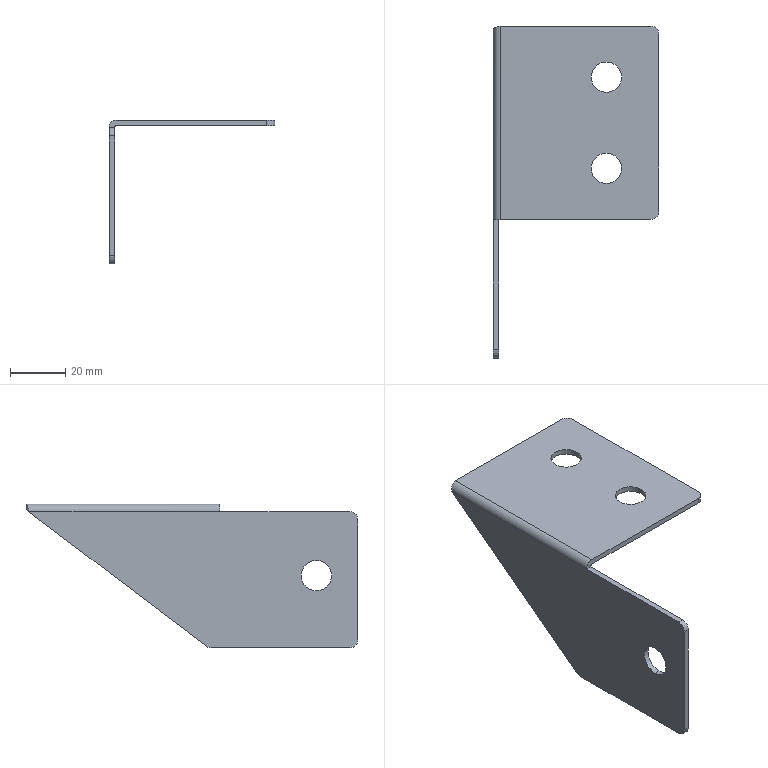Part | SolidWorks | features BaseBody 1 | 1 solid | 25 faces | box 60 x 120 x 52 mm | volume 16335 mm3 | cylinder 13 | plane 11 | spline 1 | commonest cylinder face diameters 11 x6 6 x5 1.473 x1 5.473 x1
STEP:
#1=CARTESIAN_POINT('',(-28.,-70.,-53.368));
#2=VERTEX_POINT('',#1);
#3=CARTESIAN_POINT('',(-28.,-70.,-42.368));
#4=VERTEX_POINT('',#3);
#5=CARTESIAN_POINT('',(-28.,-70.,-47.868));
#6=DIRECTION('',(-1.,0.,0.));
#7=DIRECTION('',(0.,0.,1.));
#8=AXIS2_PLACEMENT_3D('',#5,#6,#7);
#9=CIRCLE('',#8,5.5);
#10=EDGE_CURVE('',#2,#4,#9,.T.);
#11=ORIENTED_EDGE('',*,*,#10,.F.);
#12=CARTESIAN_POINT('',(-30.,-70.,-53.368));
#13=VERTEX_POINT('',#12);
#14=CARTESIAN_POINT('',(-20.,-70.,-53.368));
#15=DIRECTION('',(-1.,0.,0.));
#16=VECTOR('',#15,1000.);
#17=LINE('',#14,#16);
#18=EDGE_CURVE('',#2,#13,#17,.T.);
#19=ORIENTED_EDGE('',*,*,#18,.T.);
#20=CARTESIAN_POINT('',(-30.,-70.,-42.368));
#21=VERTEX_POINT('',#20);
#22=CARTESIAN_POINT('',(-30.,-70.,-47.868));
#23=DIRECTION('',(1.,0.,0.));
#24=DIRECTION('',(0.,0.,1.));
#25=AXIS2_PLACEMENT_3D('',#22,#23,#24);
#26=CIRCLE('',#25,5.5);
#27=EDGE_CURVE('',#21,#13,#26,.T.);
#28=ORIENTED_EDGE('',*,*,#27,.F.);
#29=CARTESIAN_POINT('',(-20.,-70.,-42.368));
#30=DIRECTION('',(-1.,0.,0.));
#31=VECTOR('',#30,1000.);
#32=LINE('',#29,#31);
#33=EDGE_CURVE('',#4,#21,#32,.T.);
#34=ORIENTED_EDGE('',*,*,#33,.F.);
#35=EDGE_LOOP('',(#11,#19,#28,#34));
#36=FACE_OUTER_BOUND('',#35,.T.);
#37=CARTESIAN_POINT('',(-20.,-70.,-47.868));
#38=DIRECTION('',(-1.,0.,0.));
#39=DIRECTION('',(0.,0.,1.));
#40=AXIS2_PLACEMENT_3D('',#37,#38,#39);
#41=CYLINDRICAL_SURFACE('',#40,5.5);
#42=ADVANCED_FACE('',(#36),#41,.F.);
#43=CARTESIAN_POINT('',(16.5,16.5,-22.));
#44=VERTEX_POINT('',#43);
#45=CARTESIAN_POINT('',(5.5,16.5,-22.));
#46=VERTEX_POINT('',#45);
#47=CARTESIAN_POINT('',(11.,16.5,-22.));
#48=DIRECTION('',(0.,0.,-1.));
#49=DIRECTION('',(-1.,0.,0.));
#50=AXIS2_PLACEMENT_3D('',#47,#48,#49);
#51=CIRCLE('',#50,5.5);
#52=EDGE_CURVE('',#44,#46,#51,.T.);
#53=ORIENTED_EDGE('',*,*,#52,.F.);
#54=CARTESIAN_POINT('',(16.5,16.5,-24.));
#55=VERTEX_POINT('',#54);
#56=CARTESIAN_POINT('',(16.5,16.5,-22.));
#57=DIRECTION('',(0.,0.,-1.));
#58=VECTOR('',#57,1000.);
#59=LINE('',#56,#58);
#60=EDGE_CURVE('',#44,#55,#59,.T.);
#61=ORIENTED_EDGE('',*,*,#60,.T.);
#62=CARTESIAN_POINT('',(5.5,16.5,-24.));
#63=VERTEX_POINT('',#62);
#64=CARTESIAN_POINT('',(11.,16.5,-24.));
#65=DIRECTION('',(0.,0.,1.));
#66=DIRECTION('',(-1.,0.,0.));
#67=AXIS2_PLACEMENT_3D('',#64,#65,#66);
#68=CIRCLE('',#67,5.5);
#69=EDGE_CURVE('',#63,#55,#68,.T.);
#70=ORIENTED_EDGE('',*,*,#69,.F.);
#71=CARTESIAN_POINT('',(5.5,16.5,-22.));
#72=DIRECTION('',(0.,0.,-1.));
#73=VECTOR('',#72,1000.);
#74=LINE('',#71,#73);
#75=EDGE_CURVE('',#46,#63,#74,.T.);
#76=ORIENTED_EDGE('',*,*,#75,.F.);
#77=EDGE_LOOP('',(#53,#61,#70,#76));
#78=FACE_OUTER_BOUND('',#77,.T.);
#79=CARTESIAN_POINT('',(11.,16.5,-22.));
#80=DIRECTION('',(0.,0.,-1.));
#81=DIRECTION('',(-1.,0.,0.));
#82=AXIS2_PLACEMENT_3D('',#79,#80,#81);
#83=CYLINDRICAL_SURFACE('',#82,5.5);
#84=ADVANCED_FACE('',(#78),#83,.F.);
#85=CARTESIAN_POINT('',(16.5,-16.5,-22.));
#86=VERTEX_POINT('',#85);
#87=CARTESIAN_POINT('',(5.5,-16.5,-22.));
#88=VERTEX_POINT('',#87);
#89=CARTESIAN_POINT('',(11.,-16.5,-22.));
#90=DIRECTION('',(0.,0.,-1.));
#91=DIRECTION('',(-1.,0.,0.));
#92=AXIS2_PLACEMENT_3D('',#89,#90,#91);
#93=CIRCLE('',#92,5.5);
#94=EDGE_CURVE('',#86,#88,#93,.T.);
#95=ORIENTED_EDGE('',*,*,#94,.F.);
#96=CARTESIAN_POINT('',(16.5,-16.5,-24.));
#97=VERTEX_POINT('',#96);
#98=CARTESIAN_POINT('',(16.5,-16.5,-22.));
#99=DIRECTION('',(0.,0.,-1.));
#100=VECTOR('',#99,1000.);
#101=LINE('',#98,#100);
#102=EDGE_CURVE('',#86,#97,#101,.T.);
#103=ORIENTED_EDGE('',*,*,#102,.T.);
#104=CARTESIAN_POINT('',(5.5,-16.5,-24.));
#105=VERTEX_POINT('',#104);
#106=CARTESIAN_POINT('',(11.,-16.5,-24.));
#107=DIRECTION('',(0.,0.,1.));
#108=DIRECTION('',(-1.,0.,0.));
#109=AXIS2_PLACEMENT_3D('',#106,#107,#108);
#110=CIRCLE('',#109,5.5);
#111=EDGE_CURVE('',#105,#97,#110,.T.);
#112=ORIENTED_EDGE('',*,*,#111,.F.);
#113=CARTESIAN_POINT('',(5.5,-16.5,-22.));
#114=DIRECTION('',(0.,0.,-1.));
#115=VECTOR('',#114,1000.);
#116=LINE('',#113,#115);
#117=EDGE_CURVE('',#88,#105,#116,.T.);
#118=ORIENTED_EDGE('',*,*,#117,.F.);
#119=EDGE_LOOP('',(#95,#103,#112,#118));
#120=FACE_OUTER_BOUND('',#119,.T.);
#121=CARTESIAN_POINT('',(11.,-16.5,-22.));
#122=DIRECTION('',(0.,0.,-1.));
#123=DIRECTION('',(-1.,0.,0.));
#124=AXIS2_PLACEMENT_3D('',#121,#122,#123);
#125=CYLINDRICAL_SURFACE('',#124,5.5);
#126=ADVANCED_FACE('',(#120),#125,.F.);
#127=CARTESIAN_POINT('',(-30.,-32.,-74.));
#128=VERTEX_POINT('',#127);
#129=CARTESIAN_POINT('',(-30.,-82.,-74.));
#130=VERTEX_POINT('',#129);
#131=CARTESIAN_POINT('',(-30.,-32.,-74.));
#132=DIRECTION('',(0.,-1.,0.));
#133=VECTOR('',#132,1000.);
#134=LINE('',#131,#133);
#135=EDGE_CURVE('',#128,#130,#134,.T.);
#136=ORIENTED_EDGE('',*,*,#135,.T.);
#137=CARTESIAN_POINT('',(-30.,-85.,-71.));
#138=VERTEX_POINT('',#137);
#139=CARTESIAN_POINT('',(-30.,-82.,-71.));
#140=DIRECTION('',(-1.,0.,0.));
#141=DIRECTION('',(0.,0.,-1.));
#142=AXIS2_PLACEMENT_3D('',#139,#140,#141);
#143=CIRCLE('',#142,3.);
#144=EDGE_CURVE('',#130,#138,#143,.T.);
#145=ORIENTED_EDGE('',*,*,#144,.T.);
#146=CARTESIAN_POINT('',(-30.,-85.,-27.737));
#147=VERTEX_POINT('',#146);
#148=CARTESIAN_POINT('',(-30.,-85.,-71.));
#149=DIRECTION('',(0.,0.,1.));
#150=VECTOR('',#149,1000.);
#151=LINE('',#148,#150);
#152=EDGE_CURVE('',#138,#147,#151,.T.);
#153=ORIENTED_EDGE('',*,*,#152,.T.);
#154=CARTESIAN_POINT('',(-30.,-82.,-24.737));
#155=VERTEX_POINT('',#154);
#156=CARTESIAN_POINT('',(-30.,-82.,-27.737));
#157=DIRECTION('',(-1.,0.,0.));
#158=DIRECTION('',(0.,0.,-1.));
#159=AXIS2_PLACEMENT_3D('',#156,#157,#158);
#160=CIRCLE('',#159,3.);
#161=EDGE_CURVE('',#147,#155,#160,.T.);
#162=ORIENTED_EDGE('',*,*,#161,.T.);
#163=CARTESIAN_POINT('',(-30.,-35.,-24.737));
#164=VERTEX_POINT('',#163);
#165=CARTESIAN_POINT('',(-30.,-32.,-24.737));
#166=DIRECTION('',(0.,1.,0.));
#167=VECTOR('',#166,1000.);
#168=LINE('',#165,#167);
#169=EDGE_CURVE('',#155,#164,#168,.T.);
#170=ORIENTED_EDGE('',*,*,#169,.T.);
#171=CARTESIAN_POINT('',(-30.,34.028,-24.737));
#172=VERTEX_POINT('',#171);
#173=CARTESIAN_POINT('',(-30.,-32.,-24.737));
#174=DIRECTION('',(0.,1.,0.));
#175=VECTOR('',#174,1000.);
#176=LINE('',#173,#175);
#177=EDGE_CURVE('',#164,#172,#176,.T.);
#178=ORIENTED_EDGE('',*,*,#177,.T.);
#179=CARTESIAN_POINT('',(-30.,-30.188,-73.391));
#180=VERTEX_POINT('',#179);
#181=CARTESIAN_POINT('',(-30.,34.028,-24.737));
#182=DIRECTION('',(0.,-0.7971,-0.6039));
#183=VECTOR('',#182,1000.);
#184=LINE('',#181,#183);
#185=EDGE_CURVE('',#172,#180,#184,.T.);
#186=ORIENTED_EDGE('',*,*,#185,.T.);
#187=CARTESIAN_POINT('',(-30.,-32.,-71.));
#188=DIRECTION('',(-1.,0.,0.));
#189=DIRECTION('',(0.,0.,-1.));
#190=AXIS2_PLACEMENT_3D('',#187,#188,#189);
#191=CIRCLE('',#190,3.);
#192=EDGE_CURVE('',#180,#128,#191,.T.);
#193=ORIENTED_EDGE('',*,*,#192,.T.);
#194=EDGE_LOOP('',(#136,#145,#153,#162,#170,#178,#186,#193));
#195=FACE_OUTER_BOUND('',#194,.T.);
#196=ORIENTED_EDGE('',*,*,#27,.T.);
#197=CARTESIAN_POINT('',(-30.,-70.,-47.868));
#198=DIRECTION('',(1.,0.,0.));
#199=DIRECTION('',(0.,0.,1.));
#200=AXIS2_PLACEMENT_3D('',#197,#198,#199);
#201=CIRCLE('',#200,5.5);
#202=EDGE_CURVE('',#13,#21,#201,.T.);
#203=ORIENTED_EDGE('',*,*,#202,.T.);
#204=EDGE_LOOP('',(#196,#203));
#205=FACE_BOUND('',#204,.T.);
#206=CARTESIAN_POINT('',(-30.,-32.,-71.));
#207=DIRECTION('',(-1.,0.,0.));
#208=DIRECTION('',(0.,0.,1.));
#209=AXIS2_PLACEMENT_3D('',#206,#207,#208);
#210=PLANE('',#209);
#211=ADVANCED_FACE('',(#195,#205),#210,.T.);
#212=ORIENTED_EDGE('',*,*,#144,.F.);
#213=CARTESIAN_POINT('',(-28.,-82.,-74.));
#214=VERTEX_POINT('',#213);
#215=CARTESIAN_POINT('',(-30.,-82.,-74.));
#216=DIRECTION('',(1.,0.,0.));
#217=VECTOR('',#216,1000.);
#218=LINE('',#215,#217);
#219=EDGE_CURVE('',#130,#214,#218,.T.);
#220=ORIENTED_EDGE('',*,*,#219,.T.);
#221=CARTESIAN_POINT('',(-28.,-85.,-71.));
#222=VERTEX_POINT('',#221);
#223=CARTESIAN_POINT('',(-28.,-82.,-71.));
#224=DIRECTION('',(-1.,0.,0.));
#225=DIRECTION('',(0.,0.,-1.));
#226=AXIS2_PLACEMENT_3D('',#223,#224,#225);
#227=CIRCLE('',#226,3.);
#228=EDGE_CURVE('',#214,#222,#227,.T.);
#229=ORIENTED_EDGE('',*,*,#228,.T.);
#230=CARTESIAN_POINT('',(-30.,-85.,-71.));
#231=DIRECTION('',(-1.,0.,0.));
#232=VECTOR('',#231,1000.);
#233=LINE('',#230,#232);
#234=EDGE_CURVE('',#222,#138,#233,.T.);
#235=ORIENTED_EDGE('',*,*,#234,.T.);
#236=EDGE_LOOP('',(#212,#220,#229,#235));
#237=FACE_OUTER_BOUND('',#236,.T.);
#238=CARTESIAN_POINT('',(-30.,-82.,-71.));
#239=DIRECTION('',(1.,0.,0.));
#240=DIRECTION('',(0.,0.,-1.));
#241=AXIS2_PLACEMENT_3D('',#238,#239,#240);
#242=CYLINDRICAL_SURFACE('',#241,3.);
#243=ADVANCED_FACE('',(#237),#242,.T.);
#244=ORIENTED_EDGE('',*,*,#219,.F.);
#245=ORIENTED_EDGE('',*,*,#135,.F.);
#246=CARTESIAN_POINT('',(-28.,-32.,-74.));
#247=VERTEX_POINT('',#246);
#248=CARTESIAN_POINT('',(-30.,-32.,-74.));
#249=DIRECTION('',(-1.,0.,0.));
#250=VECTOR('',#249,1000.);
#251=LINE('',#248,#250);
#252=EDGE_CURVE('',#247,#128,#251,.T.);
#253=ORIENTED_EDGE('',*,*,#252,.F.);
#254=CARTESIAN_POINT('',(-28.,-32.,-74.));
#255=DIRECTION('',(0.,1.,0.));
#256=VECTOR('',#255,1000.);
#257=LINE('',#254,#256);
#258=EDGE_CURVE('',#214,#247,#257,.T.);
#259=ORIENTED_EDGE('',*,*,#258,.F.);
#260=EDGE_LOOP('',(#244,#245,#253,#259));
#261=FACE_OUTER_BOUND('',#260,.T.);
#262=CARTESIAN_POINT('',(-30.,-32.,-74.));
#263=DIRECTION('',(0.,0.,1.));
#264=DIRECTION('',(1.,0.,0.));
#265=AXIS2_PLACEMENT_3D('',#262,#263,#264);
#266=PLANE('',#265);
#267=ADVANCED_FACE('',(#261),#266,.F.);
#268=ORIENTED_EDGE('',*,*,#192,.F.);
#269=CARTESIAN_POINT('',(-28.,-30.188,-73.391));
#270=VERTEX_POINT('',#269);
#271=CARTESIAN_POINT('',(-30.,-30.188,-73.391));
#272=DIRECTION('',(1.,0.,0.));
#273=VECTOR('',#272,1000.);
#274=LINE('',#271,#273);
#275=EDGE_CURVE('',#180,#270,#274,.T.);
#276=ORIENTED_EDGE('',*,*,#275,.T.);
#277=CARTESIAN_POINT('',(-28.,-32.,-71.));
#278=DIRECTION('',(-1.,0.,0.));
#279=DIRECTION('',(0.,0.,-1.));
#280=AXIS2_PLACEMENT_3D('',#277,#278,#279);
#281=CIRCLE('',#280,3.);
#282=EDGE_CURVE('',#270,#247,#281,.T.);
#283=ORIENTED_EDGE('',*,*,#282,.T.);
#284=ORIENTED_EDGE('',*,*,#252,.T.);
#285=EDGE_LOOP('',(#268,#276,#283,#284));
#286=FACE_OUTER_BOUND('',#285,.T.);
#287=CARTESIAN_POINT('',(-30.,-32.,-71.));
#288=DIRECTION('',(1.,0.,0.));
#289=DIRECTION('',(0.,0.,-1.));
#290=AXIS2_PLACEMENT_3D('',#287,#288,#289);
#291=CYLINDRICAL_SURFACE('',#290,3.);
#292=ADVANCED_FACE('',(#286),#291,.T.);
#293=CARTESIAN_POINT('',(-28.,34.028,-24.737));
#294=VERTEX_POINT('',#293);
#295=CARTESIAN_POINT('',(-28.,35.,-24.));
#296=DIRECTION('',(0.,0.7971,0.6039));
#297=VECTOR('',#296,1000.);
#298=LINE('',#295,#297);
#299=EDGE_CURVE('',#270,#294,#298,.T.);
#300=ORIENTED_EDGE('',*,*,#299,.F.);
#301=ORIENTED_EDGE('',*,*,#275,.F.);
#302=ORIENTED_EDGE('',*,*,#185,.F.);
#303=CARTESIAN_POINT('',(-30.,34.028,-24.737));
#304=DIRECTION('',(-1.,0.,0.));
#305=VECTOR('',#304,1000.);
#306=LINE('',#303,#305);
#307=EDGE_CURVE('',#294,#172,#306,.T.);
#308=ORIENTED_EDGE('',*,*,#307,.F.);
#309=EDGE_LOOP('',(#300,#301,#302,#308));
#310=FACE_OUTER_BOUND('',#309,.T.);
#311=CARTESIAN_POINT('',(-30.,35.,-24.));
#312=DIRECTION('',(0.,-0.6039,0.7971));
#313=DIRECTION('',(0.,-0.7971,-0.6039));
#314=AXIS2_PLACEMENT_3D('',#311,#312,#313);
#315=PLANE('',#314);
#316=ADVANCED_FACE('',(#310),#315,.F.);
#317=ORIENTED_EDGE('',*,*,#177,.F.);
#318=CARTESIAN_POINT('',(-27.263,-35.,-22.));
#319=VERTEX_POINT('',#318);
#320=CARTESIAN_POINT('',(-27.263,-35.,-24.737));
#321=DIRECTION('',(0.,1.,0.));
#322=DIRECTION('',(0.,0.,-1.));
#323=AXIS2_PLACEMENT_3D('',#320,#321,#322);
#324=CIRCLE('',#323,2.737);
#325=EDGE_CURVE('',#164,#319,#324,.T.);
#326=ORIENTED_EDGE('',*,*,#325,.T.);
#327=CARTESIAN_POINT('',(-27.263,35.,-22.));
#328=VERTEX_POINT('',#327);
#329=CARTESIAN_POINT('',(-27.263,-35.,-22.));
#330=DIRECTION('',(0.,1.,0.));
#331=VECTOR('',#330,1000.);
#332=LINE('',#329,#331);
#333=EDGE_CURVE('',#319,#328,#332,.T.);
#334=ORIENTED_EDGE('',*,*,#333,.T.);
#335=CARTESIAN_POINT('',(-27.263,35.,-22.));
#336=CARTESIAN_POINT('',(-27.625,34.918,-22.));
#337=CARTESIAN_POINT('',(-27.976,34.839,-22.07));
#338=CARTESIAN_POINT('',(-28.476,34.717,-22.277));
#339=CARTESIAN_POINT('',(-28.633,34.676,-22.361));
#340=CARTESIAN_POINT('',(-28.93,34.596,-22.559));
#341=CARTESIAN_POINT('',(-29.071,34.555,-22.674));
#342=CARTESIAN_POINT('',(-29.324,34.474,-22.927));
#343=CARTESIAN_POINT('',(-29.437,34.434,-23.065));
#344=CARTESIAN_POINT('',(-29.636,34.353,-23.362));
#345=CARTESIAN_POINT('',(-29.722,34.312,-23.522));
#346=CARTESIAN_POINT('',(-29.859,34.231,-23.852));
#347=CARTESIAN_POINT('',(-29.911,34.191,-24.023));
#348=CARTESIAN_POINT('',(-29.982,34.11,-24.375));
#349=CARTESIAN_POINT('',(-30.,34.069,-24.556));
#350=CARTESIAN_POINT('',(-30.,34.028,-24.737));
#351=B_SPLINE_CURVE_WITH_KNOTS('',3,(#335,#336,#337,#338,#339,#340,#341,#342,#343,#344,#345,#346,#347,#348,#349,#350),.UNSPECIFIED.,.F.,.F.,(4,2,2,2,2,2,2,4),(0.,0.001093,0.00164,0.002187,0.002734,0.00328,0.003827,0.004374),.UNSPECIFIED.);
#352=EDGE_CURVE('',#328,#172,#351,.T.);
#353=ORIENTED_EDGE('',*,*,#352,.T.);
#354=EDGE_LOOP('',(#317,#326,#334,#353));
#355=FACE_OUTER_BOUND('',#354,.T.);
#356=CARTESIAN_POINT('',(-27.263,-35.,-24.737));
#357=DIRECTION('',(0.,-1.,0.));
#358=DIRECTION('',(0.,0.,-1.));
#359=AXIS2_PLACEMENT_3D('',#356,#357,#358);
#360=CYLINDRICAL_SURFACE('',#359,2.737);
#361=ADVANCED_FACE('',(#355),#360,.T.);
#362=CARTESIAN_POINT('',(-28.,-82.,-24.737));
#363=VERTEX_POINT('',#362);
#364=CARTESIAN_POINT('',(-28.,-35.,-24.737));
#365=VERTEX_POINT('',#364);
#366=CARTESIAN_POINT('',(-28.,34.028,-24.737));
#367=DIRECTION('',(0.,1.,0.));
#368=VECTOR('',#367,1000.);
#369=LINE('',#366,#368);
#370=EDGE_CURVE('',#363,#365,#369,.T.);
#371=ORIENTED_EDGE('',*,*,#370,.T.);
#372=CARTESIAN_POINT('',(-28.,-35.,-24.737));
#373=DIRECTION('',(-1.,0.,0.));
#374=VECTOR('',#373,1000.);
#375=LINE('',#372,#374);
#376=EDGE_CURVE('',#365,#164,#375,.T.);
#377=ORIENTED_EDGE('',*,*,#376,.T.);
#378=ORIENTED_EDGE('',*,*,#169,.F.);
#379=CARTESIAN_POINT('',(-28.,-82.,-24.737));
#380=DIRECTION('',(1.,0.,0.));
#381=VECTOR('',#380,1000.);
#382=LINE('',#379,#381);
#383=EDGE_CURVE('',#155,#363,#382,.T.);
#384=ORIENTED_EDGE('',*,*,#383,.T.);
#385=EDGE_LOOP('',(#371,#377,#378,#384));
#386=FACE_OUTER_BOUND('',#385,.T.);
#387=CARTESIAN_POINT('',(-28.,34.028,-24.737));
#388=DIRECTION('',(0.,0.,1.));
#389=DIRECTION('',(1.,0.,0.));
#390=AXIS2_PLACEMENT_3D('',#387,#388,#389);
#391=PLANE('',#390);
#392=ADVANCED_FACE('',(#386),#391,.T.);
#393=ORIENTED_EDGE('',*,*,#161,.F.);
#394=CARTESIAN_POINT('',(-28.,-85.,-27.737));
#395=VERTEX_POINT('',#394);
#396=CARTESIAN_POINT('',(-30.,-85.,-27.737));
#397=DIRECTION('',(1.,0.,0.));
#398=VECTOR('',#397,1000.);
#399=LINE('',#396,#398);
#400=EDGE_CURVE('',#147,#395,#399,.T.);
#401=ORIENTED_EDGE('',*,*,#400,.T.);
#402=CARTESIAN_POINT('',(-28.,-82.,-27.737));
#403=DIRECTION('',(-1.,0.,0.));
#404=DIRECTION('',(0.,0.,-1.));
#405=AXIS2_PLACEMENT_3D('',#402,#403,#404);
#406=CIRCLE('',#405,3.);
#407=EDGE_CURVE('',#395,#363,#406,.T.);
#408=ORIENTED_EDGE('',*,*,#407,.T.);
#409=ORIENTED_EDGE('',*,*,#383,.F.);
#410=EDGE_LOOP('',(#393,#401,#408,#409));
#411=FACE_OUTER_BOUND('',#410,.T.);
#412=CARTESIAN_POINT('',(-30.,-82.,-27.737));
#413=DIRECTION('',(1.,0.,0.));
#414=DIRECTION('',(0.,0.,-1.));
#415=AXIS2_PLACEMENT_3D('',#412,#413,#414);
#416=CYLINDRICAL_SURFACE('',#415,3.);
#417=ADVANCED_FACE('',(#411),#416,.T.);
#418=ORIENTED_EDGE('',*,*,#400,.F.);
#419=ORIENTED_EDGE('',*,*,#152,.F.);
#420=ORIENTED_EDGE('',*,*,#234,.F.);
#421=CARTESIAN_POINT('',(-28.,-85.,-71.));
#422=DIRECTION('',(0.,0.,-1.));
#423=VECTOR('',#422,1000.);
#424=LINE('',#421,#423);
#425=EDGE_CURVE('',#395,#222,#424,.T.);
#426=ORIENTED_EDGE('',*,*,#425,.F.);
#427=EDGE_LOOP('',(#418,#419,#420,#426));
#428=FACE_OUTER_BOUND('',#427,.T.);
#429=CARTESIAN_POINT('',(-30.,-85.,-71.));
#430=DIRECTION('',(0.,1.,0.));
#431=DIRECTION('',(0.,0.,1.));
#432=AXIS2_PLACEMENT_3D('',#429,#430,#431);
#433=PLANE('',#432);
#434=ADVANCED_FACE('',(#428),#433,.F.);
#435=ORIENTED_EDGE('',*,*,#18,.F.);
#436=CARTESIAN_POINT('',(-28.,-70.,-47.868));
#437=DIRECTION('',(-1.,0.,0.));
#438=DIRECTION('',(0.,0.,1.));
#439=AXIS2_PLACEMENT_3D('',#436,#437,#438);
#440=CIRCLE('',#439,5.5);
#441=EDGE_CURVE('',#4,#2,#440,.T.);
#442=ORIENTED_EDGE('',*,*,#441,.F.);
#443=ORIENTED_EDGE('',*,*,#33,.T.);
#444=ORIENTED_EDGE('',*,*,#202,.F.);
#445=EDGE_LOOP('',(#435,#442,#443,#444));
#446=FACE_OUTER_BOUND('',#445,.T.);
#447=CARTESIAN_POINT('',(-20.,-70.,-47.868));
#448=DIRECTION('',(-1.,0.,0.));
#449=DIRECTION('',(0.,0.,1.));
#450=AXIS2_PLACEMENT_3D('',#447,#448,#449);
#451=CYLINDRICAL_SURFACE('',#450,5.5);
#452=ADVANCED_FACE('',(#446),#451,.F.);
#453=ORIENTED_EDGE('',*,*,#407,.F.);
#454=ORIENTED_EDGE('',*,*,#425,.T.);
#455=ORIENTED_EDGE('',*,*,#228,.F.);
#456=ORIENTED_EDGE('',*,*,#258,.T.);
#457=ORIENTED_EDGE('',*,*,#282,.F.);
#458=ORIENTED_EDGE('',*,*,#299,.T.);
#459=CARTESIAN_POINT('',(-28.,-32.,-24.737));
#460=DIRECTION('',(0.,1.,0.));
#461=VECTOR('',#460,1000.);
#462=LINE('',#459,#461);
#463=EDGE_CURVE('',#365,#294,#462,.T.);
#464=ORIENTED_EDGE('',*,*,#463,.F.);
#465=ORIENTED_EDGE('',*,*,#370,.F.);
#466=EDGE_LOOP('',(#453,#454,#455,#456,#457,#458,#464,#465));
#467=FACE_OUTER_BOUND('',#466,.T.);
#468=ORIENTED_EDGE('',*,*,#441,.T.);
#469=ORIENTED_EDGE('',*,*,#10,.T.);
#470=EDGE_LOOP('',(#468,#469));
#471=FACE_BOUND('',#470,.T.);
#472=CARTESIAN_POINT('',(-28.,-32.,-71.));
#473=DIRECTION('',(-1.,0.,0.));
#474=DIRECTION('',(0.,0.,1.));
#475=AXIS2_PLACEMENT_3D('',#472,#473,#474);
#476=PLANE('',#475);
#477=ADVANCED_FACE('',(#467,#471),#476,.F.);
#478=CARTESIAN_POINT('',(-27.263,35.,-24.));
#479=VERTEX_POINT('',#478);
#480=CARTESIAN_POINT('',(-27.263,35.,-23.));
#481=DIRECTION('',(0.,0.,-1.));
#482=VECTOR('',#481,1000.);
#483=LINE('',#480,#482);
#484=EDGE_CURVE('',#328,#479,#483,.T.);
#485=ORIENTED_EDGE('',*,*,#484,.T.);
#486=CARTESIAN_POINT('',(-27.263,35.,-24.));
#487=CARTESIAN_POINT('',(-27.458,34.837,-24.));
#488=CARTESIAN_POINT('',(-27.647,34.677,-24.079));
#489=CARTESIAN_POINT('',(-27.921,34.352,-24.352));
#490=CARTESIAN_POINT('',(-28.,34.191,-24.542));
#491=CARTESIAN_POINT('',(-28.,34.028,-24.737));
#492=B_SPLINE_CURVE_WITH_KNOTS('',3,(#486,#487,#488,#489,#490,#491),.UNSPECIFIED.,.F.,.F.,(4,2,4),(0.,0.0007533,0.001507),.UNSPECIFIED.);
#493=EDGE_CURVE('',#479,#294,#492,.T.);
#494=ORIENTED_EDGE('',*,*,#493,.T.);
#495=ORIENTED_EDGE('',*,*,#307,.T.);
#496=ORIENTED_EDGE('',*,*,#352,.F.);
#497=EDGE_LOOP('',(#485,#494,#495,#496));
#498=FACE_OUTER_BOUND('',#497,.T.);
#499=CARTESIAN_POINT('',(-27.263,35.,-21.98));
#500=CARTESIAN_POINT('',(-27.624,34.919,-21.98));
#501=CARTESIAN_POINT('',(-27.985,34.838,-22.052));
#502=CARTESIAN_POINT('',(-28.652,34.676,-22.328));
#503=CARTESIAN_POINT('',(-28.957,34.595,-22.532));
#504=CARTESIAN_POINT('',(-29.468,34.433,-23.043));
#505=CARTESIAN_POINT('',(-29.672,34.352,-23.348));
#506=CARTESIAN_POINT('',(-29.948,34.19,-24.015));
#507=CARTESIAN_POINT('',(-30.02,34.109,-24.376));
#508=CARTESIAN_POINT('',(-30.02,34.028,-24.737));
#509=CARTESIAN_POINT('',(-27.263,35.,-22.));
#510=CARTESIAN_POINT('',(-27.622,34.919,-22.));
#511=CARTESIAN_POINT('',(-27.98,34.838,-22.071));
#512=CARTESIAN_POINT('',(-28.642,34.676,-22.345));
#513=CARTESIAN_POINT('',(-28.945,34.595,-22.548));
#514=CARTESIAN_POINT('',(-29.452,34.433,-23.055));
#515=CARTESIAN_POINT('',(-29.655,34.352,-23.358));
#516=CARTESIAN_POINT('',(-29.929,34.19,-24.02));
#517=CARTESIAN_POINT('',(-30.,34.109,-24.378));
#518=CARTESIAN_POINT('',(-30.,34.028,-24.737));
#519=CARTESIAN_POINT('',(-27.263,35.,-24.));
#520=CARTESIAN_POINT('',(-27.36,34.919,-24.));
#521=CARTESIAN_POINT('',(-27.456,34.838,-24.019));
#522=CARTESIAN_POINT('',(-27.634,34.676,-24.093));
#523=CARTESIAN_POINT('',(-27.716,34.595,-24.148));
#524=CARTESIAN_POINT('',(-27.852,34.433,-24.284));
#525=CARTESIAN_POINT('',(-27.907,34.352,-24.366));
#526=CARTESIAN_POINT('',(-27.981,34.19,-24.544));
#527=CARTESIAN_POINT('',(-28.,34.109,-24.64));
#528=CARTESIAN_POINT('',(-28.,34.028,-24.737));
#529=CARTESIAN_POINT('',(-27.263,35.,-24.02));
#530=CARTESIAN_POINT('',(-27.357,34.919,-24.02));
#531=CARTESIAN_POINT('',(-27.451,34.838,-24.039));
#532=CARTESIAN_POINT('',(-27.624,34.676,-24.111));
#533=CARTESIAN_POINT('',(-27.704,34.595,-24.164));
#534=CARTESIAN_POINT('',(-27.836,34.433,-24.296));
#535=CARTESIAN_POINT('',(-27.889,34.352,-24.376));
#536=CARTESIAN_POINT('',(-27.961,34.19,-24.549));
#537=CARTESIAN_POINT('',(-27.98,34.109,-24.643));
#538=CARTESIAN_POINT('',(-27.98,34.028,-24.737));
#539=B_SPLINE_SURFACE_WITH_KNOTS('',1,3,((#499,#500,#501,#502,#503,#504,#505,#506,#507,#508),(#509,#510,#511,#512,#513,#514,#515,#516,#517,#518),(#519,#520,#521,#522,#523,#524,#525,#526,#527,#528),(#529,#530,#531,#532,#533,#534,#535,#536,#537,#538)),.UNSPECIFIED.,.F.,.F.,.F.,(2,1,1,2),(4,2,2,2,4),(-0.01,0.,1.,1.01),(0.,0.25,0.5,0.75,1.),.UNSPECIFIED.);
#540=ADVANCED_FACE('',(#498),#539,.T.);
#541=CARTESIAN_POINT('',(-27.263,-35.,-24.));
#542=VERTEX_POINT('',#541);
#543=CARTESIAN_POINT('',(-27.263,-35.,-24.737));
#544=DIRECTION('',(0.,-1.,0.));
#545=DIRECTION('',(0.,0.,-1.));
#546=AXIS2_PLACEMENT_3D('',#543,#544,#545);
#547=CIRCLE('',#546,0.7366);
#548=EDGE_CURVE('',#542,#365,#547,.T.);
#549=ORIENTED_EDGE('',*,*,#548,.F.);
#550=CARTESIAN_POINT('',(27.,-35.,-24.));
#551=VERTEX_POINT('',#550);
#552=CARTESIAN_POINT('',(-30.,-35.,-24.));
#553=DIRECTION('',(1.,0.,0.));
#554=VECTOR('',#553,1000.);
#555=LINE('',#552,#554);
#556=EDGE_CURVE('',#542,#551,#555,.T.);
#557=ORIENTED_EDGE('',*,*,#556,.T.);
#558=CARTESIAN_POINT('',(27.,-35.,-22.));
#559=VERTEX_POINT('',#558);
#560=CARTESIAN_POINT('',(27.,-35.,-22.));
#561=DIRECTION('',(0.,0.,1.));
#562=VECTOR('',#561,1000.);
#563=LINE('',#560,#562);
#564=EDGE_CURVE('',#551,#559,#563,.T.);
#565=ORIENTED_EDGE('',*,*,#564,.T.);
#566=CARTESIAN_POINT('',(0.,-35.,-22.));
#567=DIRECTION('',(1.,0.,0.));
#568=VECTOR('',#567,1000.);
#569=LINE('',#566,#568);
#570=EDGE_CURVE('',#319,#559,#569,.T.);
#571=ORIENTED_EDGE('',*,*,#570,.F.);
#572=ORIENTED_EDGE('',*,*,#325,.F.);
#573=ORIENTED_EDGE('',*,*,#376,.F.);
#574=EDGE_LOOP('',(#549,#557,#565,#571,#572,#573));
#575=FACE_OUTER_BOUND('',#574,.T.);
#576=CARTESIAN_POINT('',(-27.263,-35.,-24.737));
#577=DIRECTION('',(0.,1.,0.));
#578=DIRECTION('',(0.,0.,1.));
#579=AXIS2_PLACEMENT_3D('',#576,#577,#578);
#580=PLANE('',#579);
#581=ADVANCED_FACE('',(#575),#580,.F.);
#582=ORIENTED_EDGE('',*,*,#570,.T.);
#583=CARTESIAN_POINT('',(30.,-32.,-22.));
#584=VERTEX_POINT('',#583);
#585=CARTESIAN_POINT('',(27.,-32.,-22.));
#586=DIRECTION('',(0.,0.,1.));
#587=DIRECTION('',(-1.,0.,0.));
#588=AXIS2_PLACEMENT_3D('',#585,#586,#587);
#589=CIRCLE('',#588,3.);
#590=EDGE_CURVE('',#559,#584,#589,.T.);
#591=ORIENTED_EDGE('',*,*,#590,.T.);
#592=CARTESIAN_POINT('',(30.,32.,-22.));
#593=VERTEX_POINT('',#592);
#594=CARTESIAN_POINT('',(30.,0.,-22.));
#595=DIRECTION('',(0.,1.,0.));
#596=VECTOR('',#595,1000.);
#597=LINE('',#594,#596);
#598=EDGE_CURVE('',#584,#593,#597,.T.);
#599=ORIENTED_EDGE('',*,*,#598,.T.);
#600=CARTESIAN_POINT('',(27.,35.,-22.));
#601=VERTEX_POINT('',#600);
#602=CARTESIAN_POINT('',(27.,32.,-22.));
#603=DIRECTION('',(0.,0.,1.));
#604=DIRECTION('',(-1.,0.,0.));
#605=AXIS2_PLACEMENT_3D('',#602,#603,#604);
#606=CIRCLE('',#605,3.);
#607=EDGE_CURVE('',#593,#601,#606,.T.);
#608=ORIENTED_EDGE('',*,*,#607,.T.);
#609=CARTESIAN_POINT('',(0.,35.,-22.));
#610=DIRECTION('',(-1.,0.,0.));
#611=VECTOR('',#610,1000.);
#612=LINE('',#609,#611);
#613=EDGE_CURVE('',#601,#328,#612,.T.);
#614=ORIENTED_EDGE('',*,*,#613,.T.);
#615=ORIENTED_EDGE('',*,*,#333,.F.);
#616=EDGE_LOOP('',(#582,#591,#599,#608,#614,#615));
#617=FACE_OUTER_BOUND('',#616,.T.);
#618=CARTESIAN_POINT('',(11.,16.5,-22.));
#619=DIRECTION('',(0.,0.,-1.));
#620=DIRECTION('',(-1.,0.,0.));
#621=AXIS2_PLACEMENT_3D('',#618,#619,#620);
#622=CIRCLE('',#621,5.5);
#623=EDGE_CURVE('',#46,#44,#622,.T.);
#624=ORIENTED_EDGE('',*,*,#623,.T.);
#625=ORIENTED_EDGE('',*,*,#52,.T.);
#626=EDGE_LOOP('',(#624,#625));
#627=FACE_BOUND('',#626,.T.);
#628=CARTESIAN_POINT('',(11.,-16.5,-22.));
#629=DIRECTION('',(0.,0.,-1.));
#630=DIRECTION('',(-1.,0.,0.));
#631=AXIS2_PLACEMENT_3D('',#628,#629,#630);
#632=CIRCLE('',#631,5.5);
#633=EDGE_CURVE('',#88,#86,#632,.T.);
#634=ORIENTED_EDGE('',*,*,#633,.T.);
#635=ORIENTED_EDGE('',*,*,#94,.T.);
#636=EDGE_LOOP('',(#634,#635));
#637=FACE_BOUND('',#636,.T.);
#638=CARTESIAN_POINT('',(0.,0.,-22.));
#639=DIRECTION('',(0.,0.,1.));
#640=DIRECTION('',(1.,0.,0.));
#641=AXIS2_PLACEMENT_3D('',#638,#639,#640);
#642=PLANE('',#641);
#643=ADVANCED_FACE('',(#617,#627,#637),#642,.T.);
#644=ORIENTED_EDGE('',*,*,#548,.T.);
#645=ORIENTED_EDGE('',*,*,#463,.T.);
#646=ORIENTED_EDGE('',*,*,#493,.F.);
#647=CARTESIAN_POINT('',(-27.263,-35.,-24.));
#648=DIRECTION('',(0.,1.,0.));
#649=VECTOR('',#648,1000.);
#650=LINE('',#647,#649);
#651=EDGE_CURVE('',#542,#479,#650,.T.);
#652=ORIENTED_EDGE('',*,*,#651,.F.);
#653=EDGE_LOOP('',(#644,#645,#646,#652));
#654=FACE_OUTER_BOUND('',#653,.T.);
#655=CARTESIAN_POINT('',(-27.263,-35.,-24.737));
#656=DIRECTION('',(0.,-1.,0.));
#657=DIRECTION('',(0.,0.,-1.));
#658=AXIS2_PLACEMENT_3D('',#655,#656,#657);
#659=CYLINDRICAL_SURFACE('',#658,0.7366);
#660=ADVANCED_FACE('',(#654),#659,.F.);
#661=CARTESIAN_POINT('',(27.,35.,-24.));
#662=VERTEX_POINT('',#661);
#663=CARTESIAN_POINT('',(-30.,35.,-24.));
#664=DIRECTION('',(-1.,0.,0.));
#665=VECTOR('',#664,1000.);
#666=LINE('',#663,#665);
#667=EDGE_CURVE('',#662,#479,#666,.T.);
#668=ORIENTED_EDGE('',*,*,#667,.T.);
#669=ORIENTED_EDGE('',*,*,#484,.F.);
#670=ORIENTED_EDGE('',*,*,#613,.F.);
#671=CARTESIAN_POINT('',(27.,35.,-22.));
#672=DIRECTION('',(0.,0.,-1.));
#673=VECTOR('',#672,1000.);
#674=LINE('',#671,#673);
#675=EDGE_CURVE('',#601,#662,#674,.T.);
#676=ORIENTED_EDGE('',*,*,#675,.T.);
#677=EDGE_LOOP('',(#668,#669,#670,#676));
#678=FACE_OUTER_BOUND('',#677,.T.);
#679=CARTESIAN_POINT('',(-30.,35.,-22.));
#680=DIRECTION('',(0.,1.,0.));
#681=DIRECTION('',(0.,0.,1.));
#682=AXIS2_PLACEMENT_3D('',#679,#680,#681);
#683=PLANE('',#682);
#684=ADVANCED_FACE('',(#678),#683,.T.);
#685=CARTESIAN_POINT('',(30.,-32.,-24.));
#686=VERTEX_POINT('',#685);
#687=CARTESIAN_POINT('',(27.,-32.,-24.));
#688=DIRECTION('',(0.,0.,1.));
#689=DIRECTION('',(-1.,0.,0.));
#690=AXIS2_PLACEMENT_3D('',#687,#688,#689);
#691=CIRCLE('',#690,3.);
#692=EDGE_CURVE('',#551,#686,#691,.T.);
#693=ORIENTED_EDGE('',*,*,#692,.T.);
#694=CARTESIAN_POINT('',(30.,-32.,-22.));
#695=DIRECTION('',(0.,0.,1.));
#696=VECTOR('',#695,1000.);
#697=LINE('',#694,#696);
#698=EDGE_CURVE('',#686,#584,#697,.T.);
#699=ORIENTED_EDGE('',*,*,#698,.T.);
#700=ORIENTED_EDGE('',*,*,#590,.F.);
#701=ORIENTED_EDGE('',*,*,#564,.F.);
#702=EDGE_LOOP('',(#693,#699,#700,#701));
#703=FACE_OUTER_BOUND('',#702,.T.);
#704=CARTESIAN_POINT('',(27.,-32.,-22.));
#705=DIRECTION('',(0.,0.,-1.));
#706=DIRECTION('',(-1.,0.,0.));
#707=AXIS2_PLACEMENT_3D('',#704,#705,#706);
#708=CYLINDRICAL_SURFACE('',#707,3.);
#709=ADVANCED_FACE('',(#703),#708,.T.);
#710=CARTESIAN_POINT('',(30.,32.,-24.));
#711=VERTEX_POINT('',#710);
#712=CARTESIAN_POINT('',(27.,32.,-24.));
#713=DIRECTION('',(0.,0.,1.));
#714=DIRECTION('',(-1.,0.,0.));
#715=AXIS2_PLACEMENT_3D('',#712,#713,#714);
#716=CIRCLE('',#715,3.);
#717=EDGE_CURVE('',#711,#662,#716,.T.);
#718=ORIENTED_EDGE('',*,*,#717,.T.);
#719=ORIENTED_EDGE('',*,*,#675,.F.);
#720=ORIENTED_EDGE('',*,*,#607,.F.);
#721=CARTESIAN_POINT('',(30.,32.,-22.));
#722=DIRECTION('',(0.,0.,-1.));
#723=VECTOR('',#722,1000.);
#724=LINE('',#721,#723);
#725=EDGE_CURVE('',#593,#711,#724,.T.);
#726=ORIENTED_EDGE('',*,*,#725,.T.);
#727=EDGE_LOOP('',(#718,#719,#720,#726));
#728=FACE_OUTER_BOUND('',#727,.T.);
#729=CARTESIAN_POINT('',(27.,32.,-22.));
#730=DIRECTION('',(0.,0.,-1.));
#731=DIRECTION('',(-1.,0.,0.));
#732=AXIS2_PLACEMENT_3D('',#729,#730,#731);
#733=CYLINDRICAL_SURFACE('',#732,3.);
#734=ADVANCED_FACE('',(#728),#733,.T.);
#735=ORIENTED_EDGE('',*,*,#598,.F.);
#736=ORIENTED_EDGE('',*,*,#698,.F.);
#737=CARTESIAN_POINT('',(30.,-35.,-24.));
#738=DIRECTION('',(0.,1.,0.));
#739=VECTOR('',#738,1000.);
#740=LINE('',#737,#739);
#741=EDGE_CURVE('',#686,#711,#740,.T.);
#742=ORIENTED_EDGE('',*,*,#741,.T.);
#743=ORIENTED_EDGE('',*,*,#725,.F.);
#744=EDGE_LOOP('',(#735,#736,#742,#743));
#745=FACE_OUTER_BOUND('',#744,.T.);
#746=CARTESIAN_POINT('',(30.,-35.,-22.));
#747=DIRECTION('',(1.,0.,0.));
#748=DIRECTION('',(0.,0.,-1.));
#749=AXIS2_PLACEMENT_3D('',#746,#747,#748);
#750=PLANE('',#749);
#751=ADVANCED_FACE('',(#745),#750,.T.);
#752=ORIENTED_EDGE('',*,*,#60,.F.);
#753=ORIENTED_EDGE('',*,*,#623,.F.);
#754=ORIENTED_EDGE('',*,*,#75,.T.);
#755=CARTESIAN_POINT('',(11.,16.5,-24.));
#756=DIRECTION('',(0.,0.,1.));
#757=DIRECTION('',(-1.,0.,0.));
#758=AXIS2_PLACEMENT_3D('',#755,#756,#757);
#759=CIRCLE('',#758,5.5);
#760=EDGE_CURVE('',#55,#63,#759,.T.);
#761=ORIENTED_EDGE('',*,*,#760,.F.);
#762=EDGE_LOOP('',(#752,#753,#754,#761));
#763=FACE_OUTER_BOUND('',#762,.T.);
#764=CARTESIAN_POINT('',(11.,16.5,-22.));
#765=DIRECTION('',(0.,0.,-1.));
#766=DIRECTION('',(-1.,0.,0.));
#767=AXIS2_PLACEMENT_3D('',#764,#765,#766);
#768=CYLINDRICAL_SURFACE('',#767,5.5);
#769=ADVANCED_FACE('',(#763),#768,.F.);
#770=ORIENTED_EDGE('',*,*,#102,.F.);
#771=ORIENTED_EDGE('',*,*,#633,.F.);
#772=ORIENTED_EDGE('',*,*,#117,.T.);
#773=CARTESIAN_POINT('',(11.,-16.5,-24.));
#774=DIRECTION('',(0.,0.,1.));
#775=DIRECTION('',(-1.,0.,0.));
#776=AXIS2_PLACEMENT_3D('',#773,#774,#775);
#777=CIRCLE('',#776,5.5);
#778=EDGE_CURVE('',#97,#105,#777,.T.);
#779=ORIENTED_EDGE('',*,*,#778,.F.);
#780=EDGE_LOOP('',(#770,#771,#772,#779));
#781=FACE_OUTER_BOUND('',#780,.T.);
#782=CARTESIAN_POINT('',(11.,-16.5,-22.));
#783=DIRECTION('',(0.,0.,-1.));
#784=DIRECTION('',(-1.,0.,0.));
#785=AXIS2_PLACEMENT_3D('',#782,#783,#784);
#786=CYLINDRICAL_SURFACE('',#785,5.5);
#787=ADVANCED_FACE('',(#781),#786,.F.);
#788=ORIENTED_EDGE('',*,*,#717,.F.);
#789=ORIENTED_EDGE('',*,*,#741,.F.);
#790=ORIENTED_EDGE('',*,*,#692,.F.);
#791=ORIENTED_EDGE('',*,*,#556,.F.);
#792=ORIENTED_EDGE('',*,*,#651,.T.);
#793=ORIENTED_EDGE('',*,*,#667,.F.);
#794=EDGE_LOOP('',(#788,#789,#790,#791,#792,#793));
#795=FACE_OUTER_BOUND('',#794,.T.);
#796=ORIENTED_EDGE('',*,*,#111,.T.);
#797=ORIENTED_EDGE('',*,*,#778,.T.);
#798=EDGE_LOOP('',(#796,#797));
#799=FACE_BOUND('',#798,.T.);
#800=ORIENTED_EDGE('',*,*,#69,.T.);
#801=ORIENTED_EDGE('',*,*,#760,.T.);
#802=EDGE_LOOP('',(#800,#801));
#803=FACE_BOUND('',#802,.T.);
#804=CARTESIAN_POINT('',(0.,0.,-24.));
#805=DIRECTION('',(0.,0.,1.));
#806=DIRECTION('',(1.,0.,0.));
#807=AXIS2_PLACEMENT_3D('',#804,#805,#806);
#808=PLANE('',#807);
#809=ADVANCED_FACE('',(#795,#799,#803),#808,.F.);
#810=CLOSED_SHELL('',(#42,#84,#126,#211,#243,#267,#292,#316,#361,#392,#417,#434,#452,#477,#540,#581,#643,#660,#684,#709,#734,#751,#769,#787,#809));
#811=MANIFOLD_SOLID_BREP('',#810);
#812=CARTESIAN_POINT('',(0.,0.,0.));
#813=DIRECTION('',(0.,0.,1.));
#814=DIRECTION('',(1.,0.,0.));
#815=AXIS2_PLACEMENT_3D('',#812,#813,#814);
#816=(LENGTH_UNIT()NAMED_UNIT(*)SI_UNIT(.MILLI.,.METRE.));
#817=UNCERTAINTY_MEASURE_WITH_UNIT(LENGTH_MEASURE(0.00001),#816,'','');
#818=(NAMED_UNIT(*)PLANE_ANGLE_UNIT()SI_UNIT($,.RADIAN.));
#819=(NAMED_UNIT(*)SI_UNIT($,.STERADIAN.)SOLID_ANGLE_UNIT());
#820=(GEOMETRIC_REPRESENTATION_CONTEXT(3)GLOBAL_UNCERTAINTY_ASSIGNED_CONTEXT((#817))GLOBAL_UNIT_ASSIGNED_CONTEXT((#816,#818,#819))REPRESENTATION_CONTEXT('',''));
#821=ADVANCED_BREP_SHAPE_REPRESENTATION('',(#811,#815),#820);